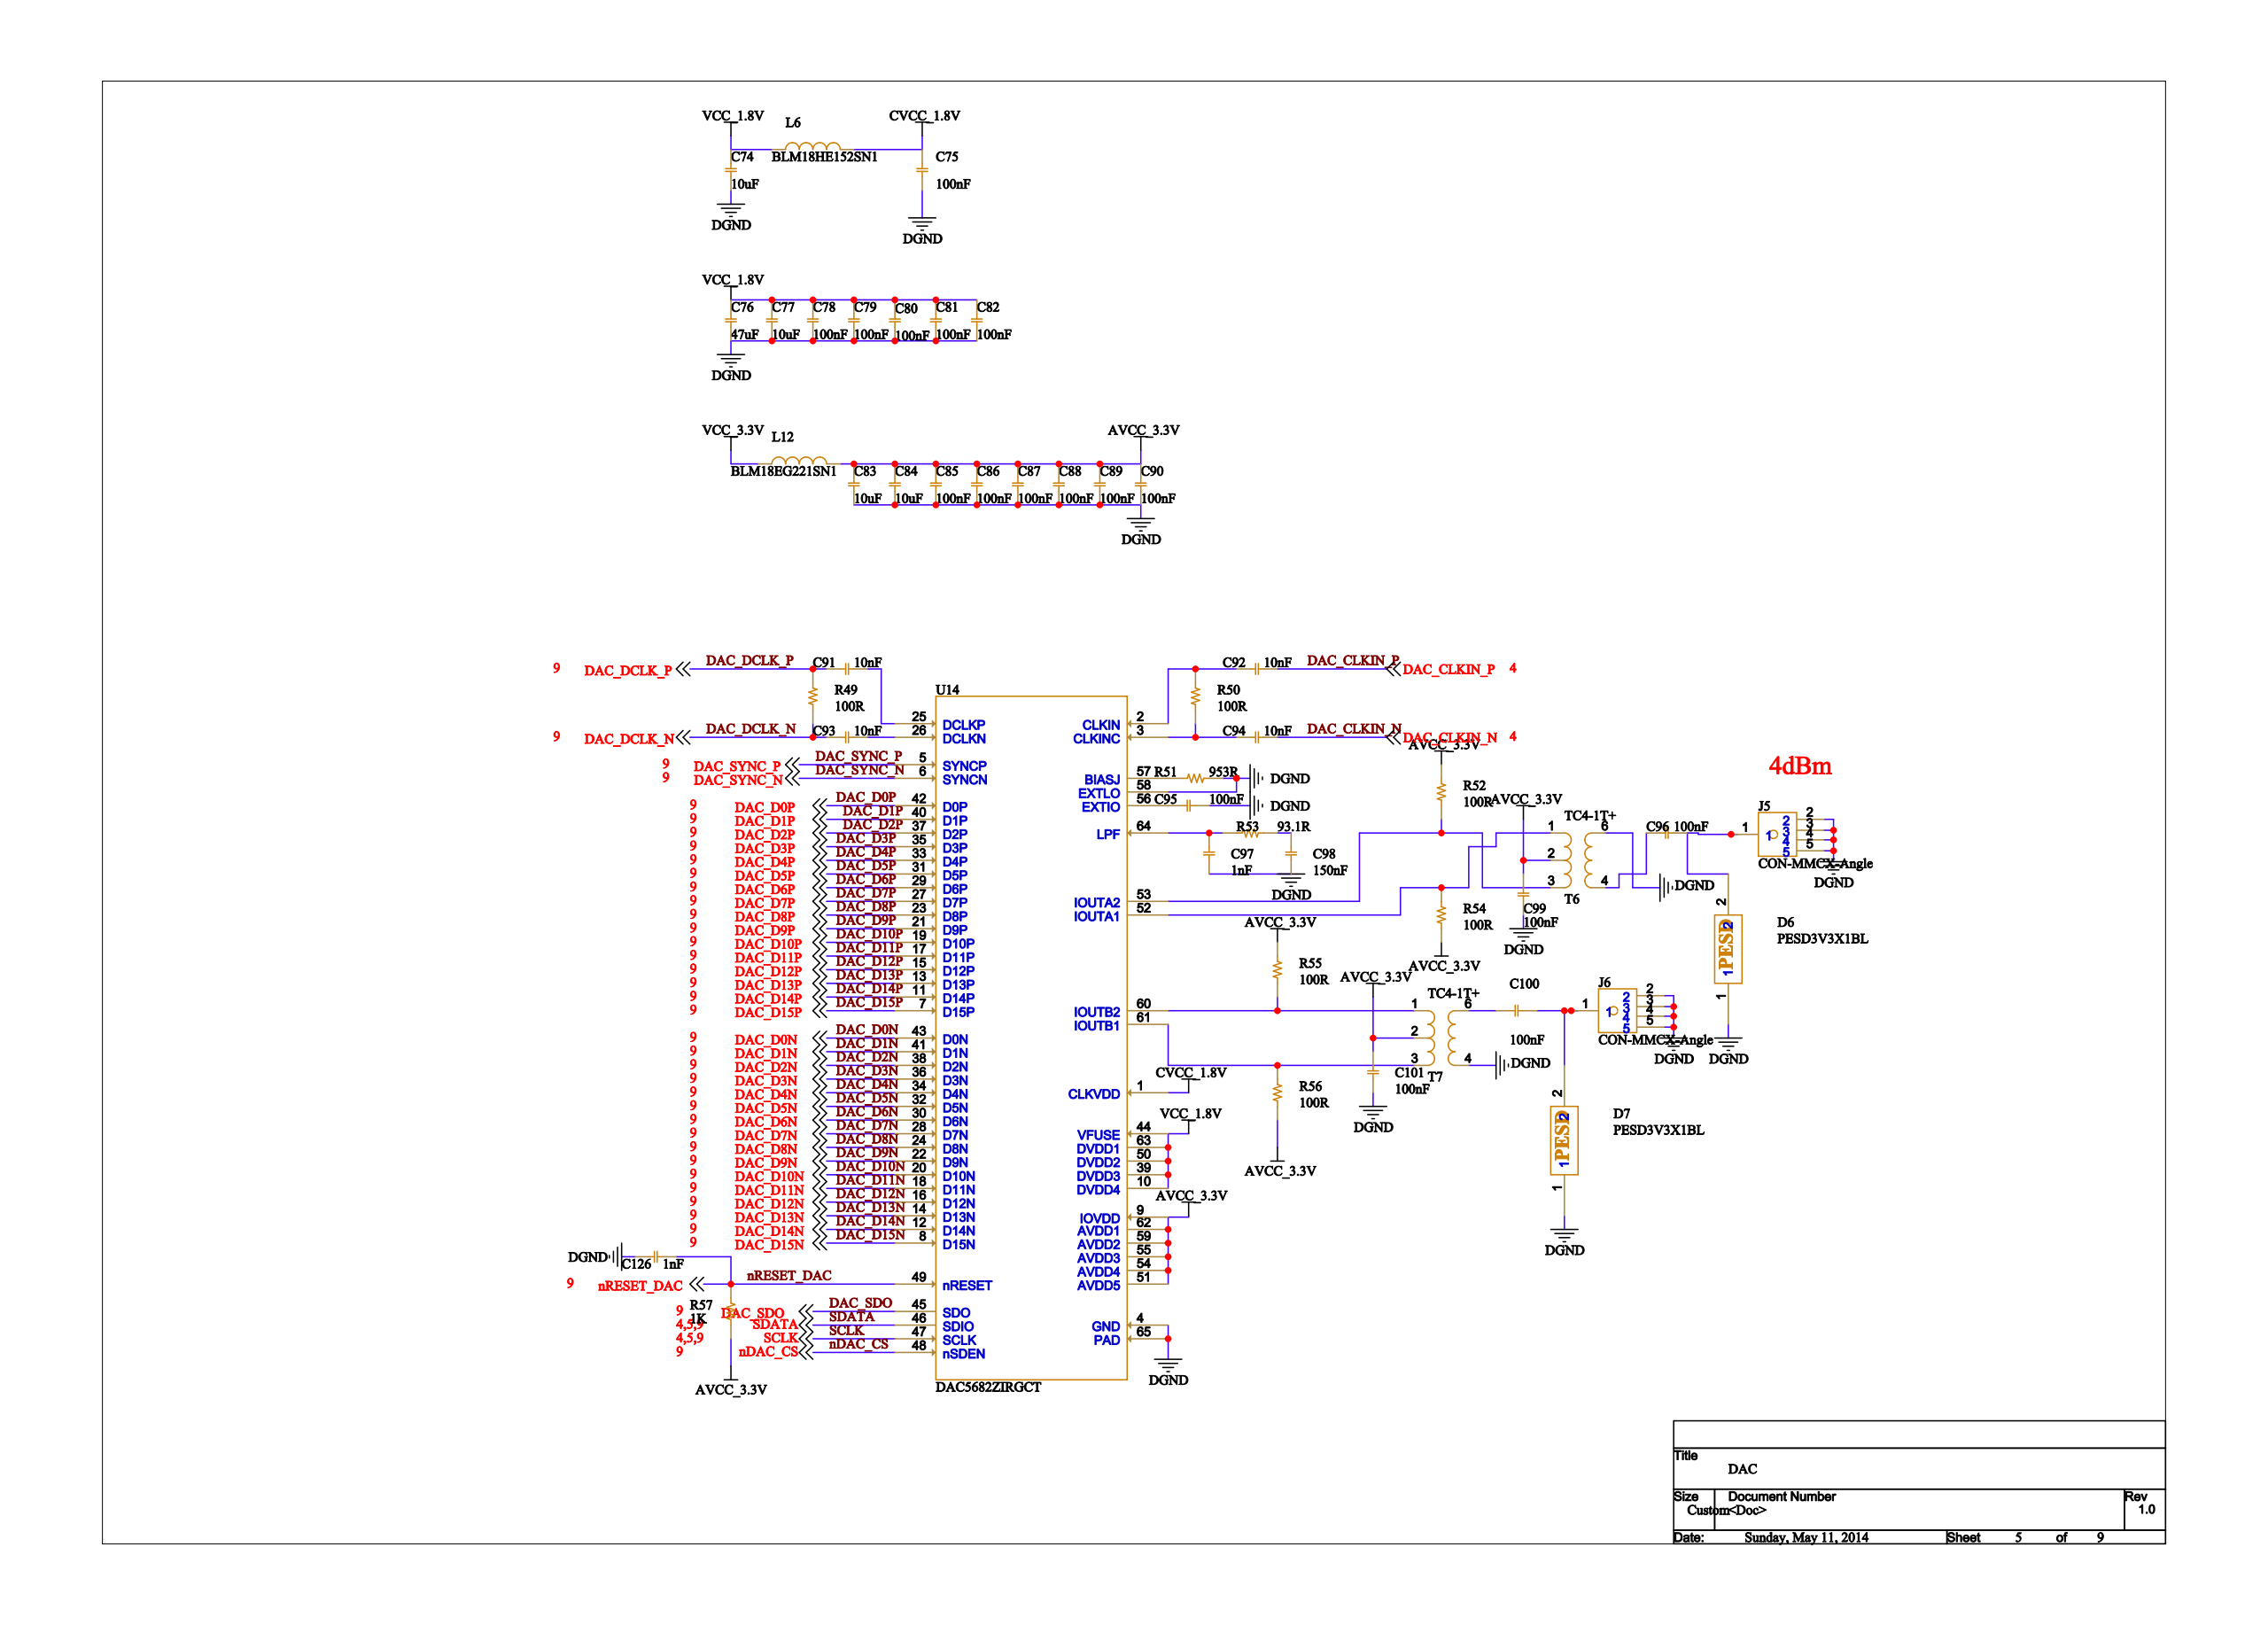Circuit board | Cadence Allegro | 233 parts | 224 nets | one sheet of the schematic
Parts on this sheet (reference | value | footprint):
C74 | 10uF | FPC-0603C
C75 | 100nF | FPC-0402C
C76 | 47uF | FPC-1206C
C77 | 10uF | FPC-0603C
C78 | 100nF | FPC-0402C
C79 | 100nF | FPC-0402C
C80 | 100nF | FPC-0402C
C81 | 100nF | FPC-0402C
C82 | 100nF | FPC-0402C
C83 | 10uF | FPC-0603C
C84 | 10uF | FPC-0603C
C85 | 100nF | FPC-0402C
C86 | 100nF | FPC-0402C
C87 | 100nF | FPC-0402C
C88 | 100nF | FPC-0402C
C89 | 100nF | FPC-0402C
C90 | 100nF | FPC-0402C
C91 | 10nF | FPC-0402C
C92 | 10nF | FPC-0402C
C93 | 10nF | FPC-0402C
C94 | 10nF | FPC-0402C
C95 | 100nF | FPC-0402C
C96 | 100nF | FPC-0402C
C97 | 1nF | FPC-0402C
C98 | 150nF | FPC-0402C
C99 | 100nF | FPC-0402C
C100 | 100nF | FPC-0402C
C101 | 100nF | FPC-0402C
C126 | 1nF | FPC-0402C
D6 | PESD3V3X1BL | SOD882
D7 | PESD3V3X1BL | SOD882
J5 | CON-MMCX-Angle | SMA
J6 | CON-MMCX-Angle | SMA
L6 | BLM18HE152SN1 | FPC-0603L
L12 | BLM18EG221SN1 | FPC-0603L
R49 | 100R | FPC-0603R
R50 | 100R | FPC-0603R
R51 | 953R | FPC-0603R
R52 | 100R | FPC-0603R
R53 | 93.1R | FPC-0603R
R54 | 100R | FPC-0603R
R55 | 100R | FPC-0603R
R56 | 100R | FPC-0603R
R57 | 1K | FPC-0603R
T6 | TC4-1T+ | FPC-TRAN5SM-3R81X3R81
T7 | TC4-1T+ | FPC-TRAN5SM-3R81X3R81
U14 | DAC5682ZIRGCT | FPC-QFN9X9-64-1
Nets of these parts (net: part-pin ...):
DGND: C74-1 C75-1 C76-2 C77-1 C78-2 C79-1 C80-1 C81-1 C82-1 C83-1 C84-1 C85-1 C86-1 C87-1 C88-1 C89-1 C90-1 C95-2 C97-1 C98-1 C99-1 C101-1 C126-2 D6-1 D7-1 J5-2 J5-3 J5-4 J5-5 J6-2 J6-3 J6-4 J6-5 R51-1 T6-6 T7-4 U14-4 U14-58 U14-65
N45660: C96-1 D6-2 J5-1
N45658: C100-1 D7-2 J6-1
N91138: C100-2 T7-6
AVCC_3.3V: C83-2 C84-2 C85-2 C86-2 C87-2 C88-2 C89-2 C90-2 C99-2 C101-2 L12-2 R52-2 R54-1 R55-2 R56-1 R57-2 T6-2 T7-2 U14-9 U14-51 U14-54 U14-55 U14-59 U14-62
VCC_3.3V: L12-1
CVCC_1.8V: C75-2 L6-2 U14-1
VCC_1.8V: C74-2 C76-1 C77-2 C78-1 C79-2 C80-2 C81-2 C82-2 L6-1 U14-10 U14-39 U14-44 U14-50 U14-63
N4598447: C95-1 U14-56
N635607: C96-2 T6-4
NRESET_DAC: C126-1 R57-1 U14-49
N45412: C97-2 R53-1 U14-64
DAC_DCLK_P: C91-1 R49-2
N00048: C91-2 U14-25
N00047: C92-1 R50-2 U14-2
DAC_CLKIN_P: C92-2
DAC_DCLK_N: C93-1 R49-1
N00052: C93-2 U14-26
N45408: C94-1 R50-1 U14-3
DAC_CLKIN_N: C94-2
N872952: C98-2 R53-2
DAC_D9N: U14-22
DAC_D9P: U14-21
DAC_SYNC_N: U14-6
DAC_SYNC_P: U14-5
DAC_D15N: U14-8
DAC_D15P: U14-7
DAC_D14N: U14-12
DAC_D14P: U14-11
DAC_D11N: U14-18
DAC_D11P: U14-17
DAC_D7N: U14-28
DAC_D7P: U14-27
DAC_D13N: U14-14
DAC_D13P: U14-13
DAC_D10N: U14-20
DAC_D10P: U14-19
DAC_D12N: U14-16
DAC_D12P: U14-15
DAC_D3N: U14-36
DAC_D3P: U14-35
DAC_D2N: U14-38
DAC_D2P: U14-37
DAC_D5N: U14-32
DAC_D5P: U14-31
DAC_D8N: U14-24
DAC_D8P: U14-23
DAC_D1N: U14-41
DAC_D1P: U14-40
DAC_D0N: U14-43
DAC_D0P: U14-42
DAC_D4N: U14-34
DAC_D4P: U14-33
DAC_D6N: U14-30
DAC_D6P: U14-29
N45484: R52-1 T6-3 U14-53
N45494: R54-2 T6-1 U14-52
N91095: R55-1 T7-1 U14-60
N00142: R56-2 T7-3 U14-61
N459845: R51-2 U14-57
SCLK: U14-47
SDATA: U14-46
DAC_SDO: U14-45